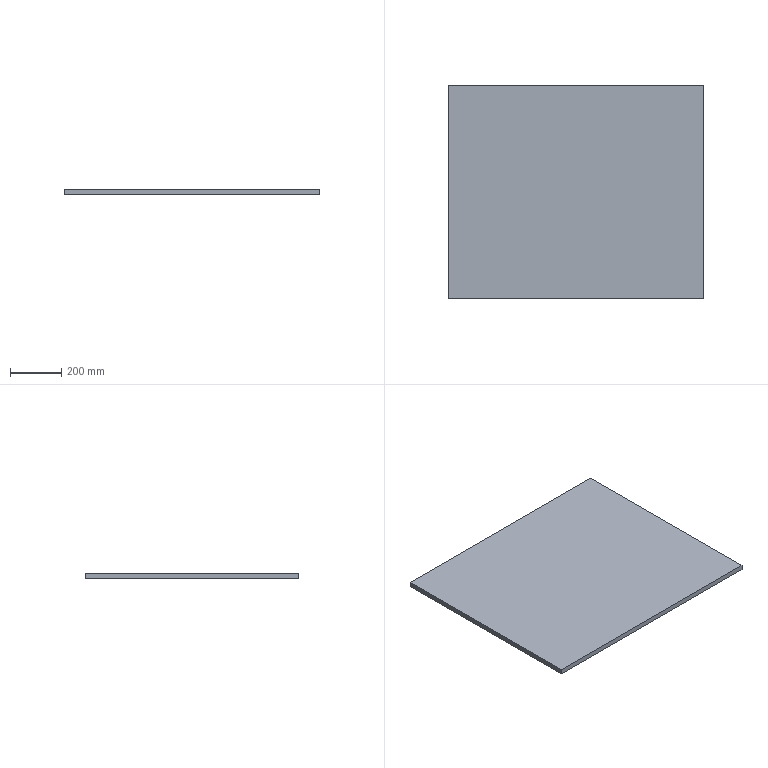Part | SolidWorks | features BaseBody 1 | 1 solid | 6 faces | box 1000 x 836 x 20 mm | volume 16720000 mm3 | plane 6
STEP:
#1=CARTESIAN_POINT('',(2687.093,2301.455,0.));
#2=VERTEX_POINT('',#1);
#3=CARTESIAN_POINT('',(2687.093,1465.455,0.));
#4=VERTEX_POINT('',#3);
#5=CARTESIAN_POINT('',(2687.093,1465.455,0.));
#6=DIRECTION('',(0.,-1.,0.));
#7=VECTOR('',#6,1000.);
#8=LINE('',#5,#7);
#9=EDGE_CURVE('',#2,#4,#8,.T.);
#10=ORIENTED_EDGE('',*,*,#9,.T.);
#11=CARTESIAN_POINT('',(2687.093,1465.455,20.));
#12=VERTEX_POINT('',#11);
#13=CARTESIAN_POINT('',(2687.093,1465.455,20.));
#14=DIRECTION('',(0.,0.,-1.));
#15=VECTOR('',#14,1000.);
#16=LINE('',#13,#15);
#17=EDGE_CURVE('',#12,#4,#16,.T.);
#18=ORIENTED_EDGE('',*,*,#17,.F.);
#19=CARTESIAN_POINT('',(2687.093,2301.455,20.));
#20=VERTEX_POINT('',#19);
#21=CARTESIAN_POINT('',(2687.093,1465.455,20.));
#22=DIRECTION('',(0.,-1.,0.));
#23=VECTOR('',#22,1000.);
#24=LINE('',#21,#23);
#25=EDGE_CURVE('',#20,#12,#24,.T.);
#26=ORIENTED_EDGE('',*,*,#25,.F.);
#27=CARTESIAN_POINT('',(2687.093,2301.455,20.));
#28=DIRECTION('',(0.,0.,-1.));
#29=VECTOR('',#28,1000.);
#30=LINE('',#27,#29);
#31=EDGE_CURVE('',#20,#2,#30,.T.);
#32=ORIENTED_EDGE('',*,*,#31,.T.);
#33=EDGE_LOOP('',(#10,#18,#26,#32));
#34=FACE_OUTER_BOUND('',#33,.T.);
#35=CARTESIAN_POINT('',(2687.093,1465.455,20.));
#36=DIRECTION('',(1.,0.,0.));
#37=DIRECTION('',(0.,1.,0.));
#38=AXIS2_PLACEMENT_3D('',#35,#36,#37);
#39=PLANE('',#38);
#40=ADVANCED_FACE('',(#34),#39,.F.);
#41=CARTESIAN_POINT('',(3687.093,1465.455,0.));
#42=VERTEX_POINT('',#41);
#43=CARTESIAN_POINT('',(3687.093,1465.455,0.));
#44=DIRECTION('',(1.,0.,0.));
#45=VECTOR('',#44,1000.);
#46=LINE('',#43,#45);
#47=EDGE_CURVE('',#4,#42,#46,.T.);
#48=ORIENTED_EDGE('',*,*,#47,.T.);
#49=CARTESIAN_POINT('',(3687.093,1465.455,20.));
#50=VERTEX_POINT('',#49);
#51=CARTESIAN_POINT('',(3687.093,1465.455,20.));
#52=DIRECTION('',(0.,0.,-1.));
#53=VECTOR('',#52,1000.);
#54=LINE('',#51,#53);
#55=EDGE_CURVE('',#50,#42,#54,.T.);
#56=ORIENTED_EDGE('',*,*,#55,.F.);
#57=CARTESIAN_POINT('',(3687.093,1465.455,20.));
#58=DIRECTION('',(1.,0.,0.));
#59=VECTOR('',#58,1000.);
#60=LINE('',#57,#59);
#61=EDGE_CURVE('',#12,#50,#60,.T.);
#62=ORIENTED_EDGE('',*,*,#61,.F.);
#63=ORIENTED_EDGE('',*,*,#17,.T.);
#64=EDGE_LOOP('',(#48,#56,#62,#63));
#65=FACE_OUTER_BOUND('',#64,.T.);
#66=CARTESIAN_POINT('',(3687.093,1465.455,20.));
#67=DIRECTION('',(0.,1.,0.));
#68=DIRECTION('',(0.,0.,1.));
#69=AXIS2_PLACEMENT_3D('',#66,#67,#68);
#70=PLANE('',#69);
#71=ADVANCED_FACE('',(#65),#70,.F.);
#72=CARTESIAN_POINT('',(3687.093,2301.455,0.));
#73=VERTEX_POINT('',#72);
#74=CARTESIAN_POINT('',(3687.093,2301.455,0.));
#75=DIRECTION('',(0.,1.,0.));
#76=VECTOR('',#75,1000.);
#77=LINE('',#74,#76);
#78=EDGE_CURVE('',#42,#73,#77,.T.);
#79=ORIENTED_EDGE('',*,*,#78,.T.);
#80=CARTESIAN_POINT('',(3687.093,2301.455,20.));
#81=VERTEX_POINT('',#80);
#82=CARTESIAN_POINT('',(3687.093,2301.455,20.));
#83=DIRECTION('',(0.,0.,-1.));
#84=VECTOR('',#83,1000.);
#85=LINE('',#82,#84);
#86=EDGE_CURVE('',#81,#73,#85,.T.);
#87=ORIENTED_EDGE('',*,*,#86,.F.);
#88=CARTESIAN_POINT('',(3687.093,2301.455,20.));
#89=DIRECTION('',(0.,1.,0.));
#90=VECTOR('',#89,1000.);
#91=LINE('',#88,#90);
#92=EDGE_CURVE('',#50,#81,#91,.T.);
#93=ORIENTED_EDGE('',*,*,#92,.F.);
#94=ORIENTED_EDGE('',*,*,#55,.T.);
#95=EDGE_LOOP('',(#79,#87,#93,#94));
#96=FACE_OUTER_BOUND('',#95,.T.);
#97=CARTESIAN_POINT('',(3687.093,2301.455,20.));
#98=DIRECTION('',(-1.,0.,0.));
#99=DIRECTION('',(0.,0.,1.));
#100=AXIS2_PLACEMENT_3D('',#97,#98,#99);
#101=PLANE('',#100);
#102=ADVANCED_FACE('',(#96),#101,.F.);
#103=CARTESIAN_POINT('',(2687.093,2301.455,0.));
#104=DIRECTION('',(-1.,0.,0.));
#105=VECTOR('',#104,1000.);
#106=LINE('',#103,#105);
#107=EDGE_CURVE('',#73,#2,#106,.T.);
#108=ORIENTED_EDGE('',*,*,#107,.T.);
#109=ORIENTED_EDGE('',*,*,#31,.F.);
#110=CARTESIAN_POINT('',(2687.093,2301.455,20.));
#111=DIRECTION('',(-1.,0.,0.));
#112=VECTOR('',#111,1000.);
#113=LINE('',#110,#112);
#114=EDGE_CURVE('',#81,#20,#113,.T.);
#115=ORIENTED_EDGE('',*,*,#114,.F.);
#116=ORIENTED_EDGE('',*,*,#86,.T.);
#117=EDGE_LOOP('',(#108,#109,#115,#116));
#118=FACE_OUTER_BOUND('',#117,.T.);
#119=CARTESIAN_POINT('',(2687.093,2301.455,20.));
#120=DIRECTION('',(0.,-1.,0.));
#121=DIRECTION('',(0.,0.,-1.));
#122=AXIS2_PLACEMENT_3D('',#119,#120,#121);
#123=PLANE('',#122);
#124=ADVANCED_FACE('',(#118),#123,.F.);
#125=ORIENTED_EDGE('',*,*,#25,.T.);
#126=ORIENTED_EDGE('',*,*,#61,.T.);
#127=ORIENTED_EDGE('',*,*,#92,.T.);
#128=ORIENTED_EDGE('',*,*,#114,.T.);
#129=EDGE_LOOP('',(#125,#126,#127,#128));
#130=FACE_OUTER_BOUND('',#129,.T.);
#131=CARTESIAN_POINT('',(0.,0.,20.));
#132=DIRECTION('',(0.,0.,-1.));
#133=DIRECTION('',(-1.,0.,0.));
#134=AXIS2_PLACEMENT_3D('',#131,#132,#133);
#135=PLANE('',#134);
#136=ADVANCED_FACE('',(#130),#135,.F.);
#137=ORIENTED_EDGE('',*,*,#9,.F.);
#138=ORIENTED_EDGE('',*,*,#107,.F.);
#139=ORIENTED_EDGE('',*,*,#78,.F.);
#140=ORIENTED_EDGE('',*,*,#47,.F.);
#141=EDGE_LOOP('',(#137,#138,#139,#140));
#142=FACE_OUTER_BOUND('',#141,.T.);
#143=CARTESIAN_POINT('',(0.,0.,0.));
#144=DIRECTION('',(0.,0.,-1.));
#145=DIRECTION('',(-1.,0.,0.));
#146=AXIS2_PLACEMENT_3D('',#143,#144,#145);
#147=PLANE('',#146);
#148=ADVANCED_FACE('',(#142),#147,.T.);
#149=CLOSED_SHELL('',(#40,#71,#102,#124,#136,#148));
#150=MANIFOLD_SOLID_BREP('',#149);
#151=CARTESIAN_POINT('',(0.,0.,0.));
#152=DIRECTION('',(0.,0.,1.));
#153=DIRECTION('',(1.,0.,0.));
#154=AXIS2_PLACEMENT_3D('',#151,#152,#153);
#155=(LENGTH_UNIT()NAMED_UNIT(*)SI_UNIT(.MILLI.,.METRE.));
#156=UNCERTAINTY_MEASURE_WITH_UNIT(LENGTH_MEASURE(0.00001),#155,'','');
#157=(NAMED_UNIT(*)PLANE_ANGLE_UNIT()SI_UNIT($,.RADIAN.));
#158=(NAMED_UNIT(*)SI_UNIT($,.STERADIAN.)SOLID_ANGLE_UNIT());
#159=(GEOMETRIC_REPRESENTATION_CONTEXT(3)GLOBAL_UNCERTAINTY_ASSIGNED_CONTEXT((#156))GLOBAL_UNIT_ASSIGNED_CONTEXT((#155,#157,#158))REPRESENTATION_CONTEXT('',''));
#160=ADVANCED_BREP_SHAPE_REPRESENTATION('',(#150,#154),#159);